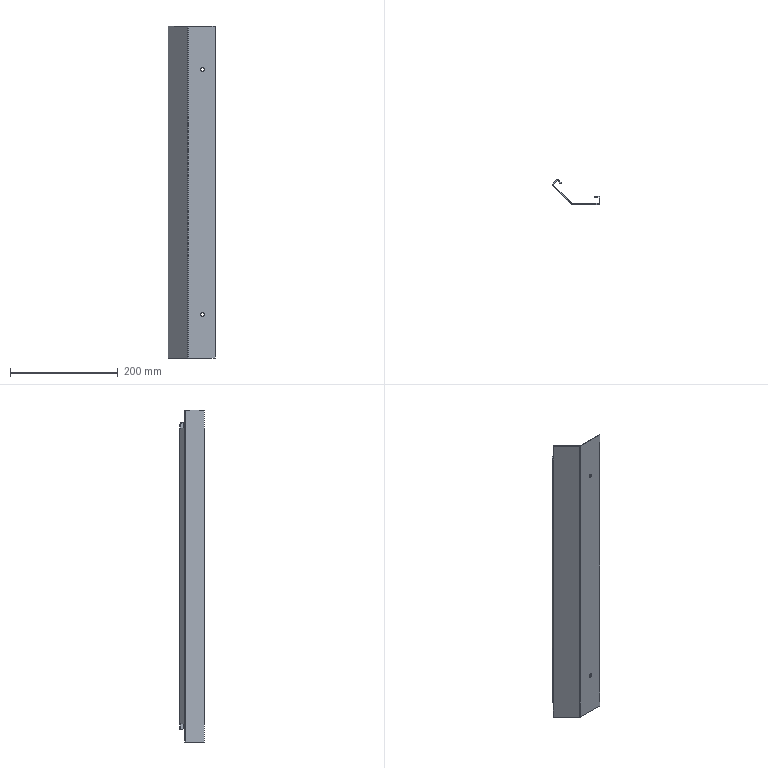Part | SolidWorks | features SMBaseFlange 3, EdgeFlange 2, Cut 1, Fillet 1, FlatPattern 1, SheetMetal 1 | 1 solid | 66 faces | box 88.831 x 46.399 x 617 mm | volume 130995 mm3 | plane 48 | cylinder 18 | commonest cylinder face diameters 0.2 x5 3.2 x5 7 x4 10 x4